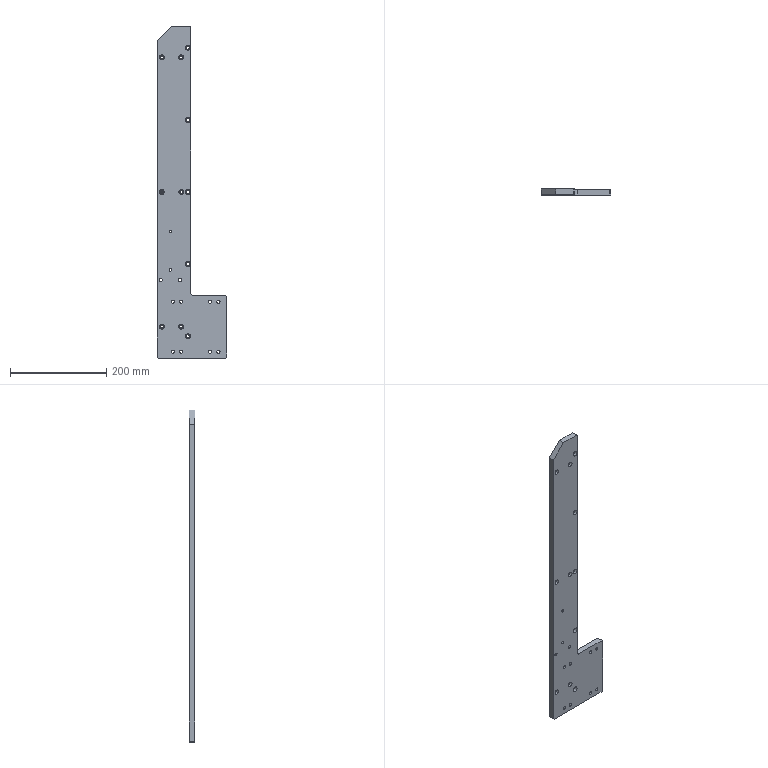Part | SolidWorks | features HoleWzd 6, Chamfer 2, Extrusion 1, ICE 1 | 1 solid | 137 faces | box 145 x 12 x 690 mm | volume 673672 mm3 | cylinder 97 | plane 36 | cone 4 | commonest cylinder face diameters 6.6 x30 11 x30 10 x17 5.5 x16 4.2 x4